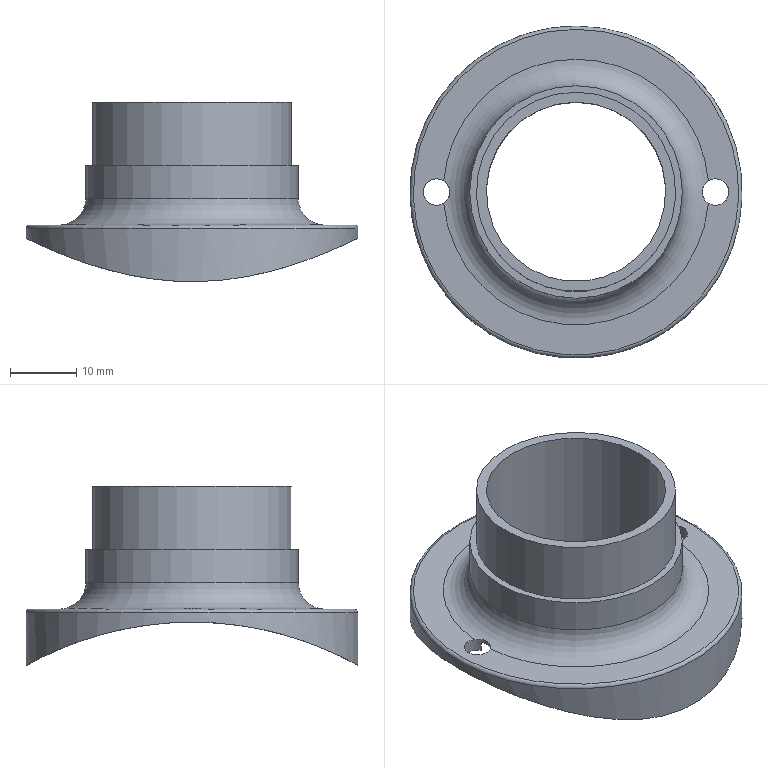Part | STEP file | 1-14.1 | 1 solid | 15 faces | box 50.002 x 50.001 x 27 mm | volume 7555 mm3 | cylinder 9 | plane 4 | torus 2 | commonest cylinder face diameters 4 x2 38.5 x2 27 x1 30 x1 32 x1 50 x1